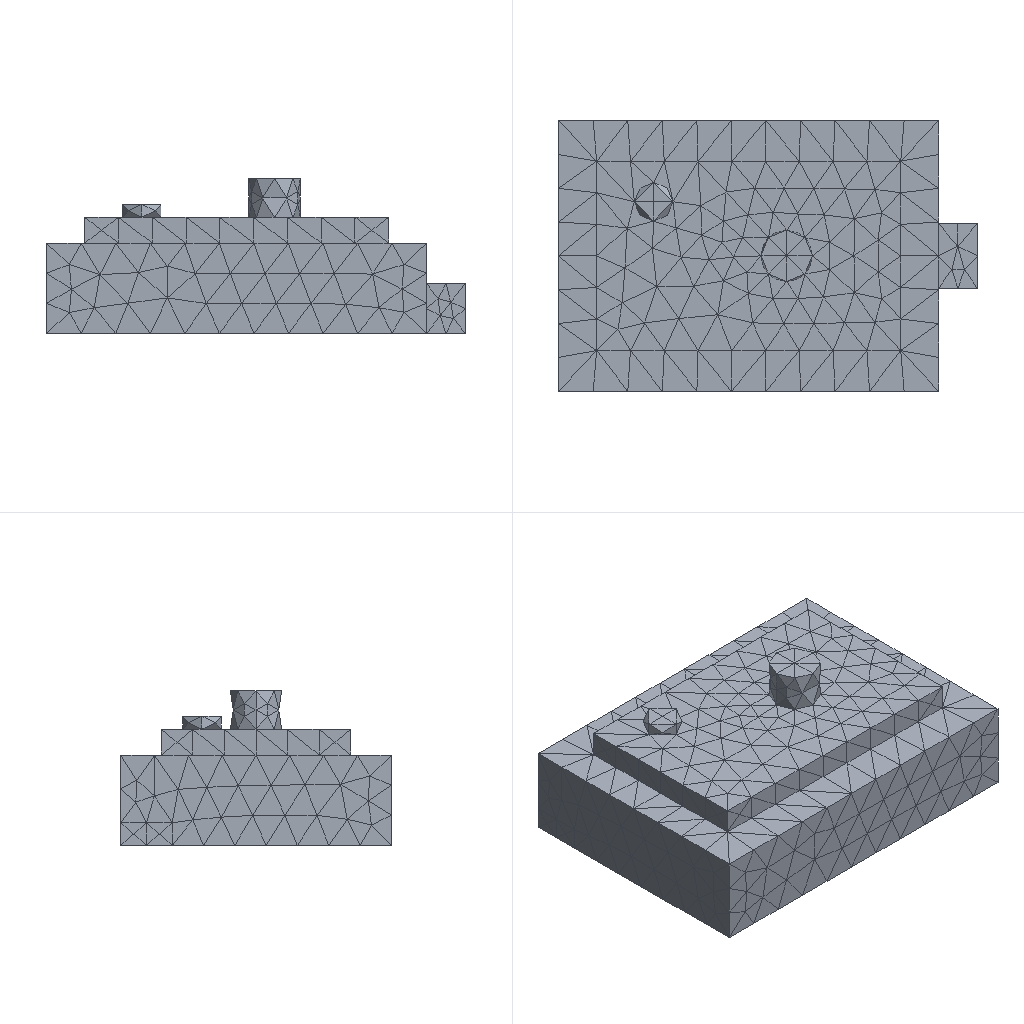Simulation study | ansys mapdl
Set-up summary:
category,name,step,type,value,unit,region
solver,ansys_mapdl
units,mm-N-s-tonne (MPa),,inferred,E=210000 density=
analysis,model,,static
mesh,nodes,,,5151
mesh,elements,,,3114
element_type,SOLID187,,,3114
material,mat 1,,E,210000
material,mat 1,,nu,0.3
load,,model,body load temp,,,all
load,,model,force,"1000 [dir=(0, 0, -1) n=162]",,node list
bc,,model,fixed,"[dofs=UX,UY,UZ n=5109]",,node list
Ansys APDL input file, long lists of numbers shortened:
/COM,ANSYS RELEASE 2026 R1           BUILD 26.1      UP20260202       09:08:46
/PREP7
/NOPR
/TITLE,2
ANTYPE, 0
*IF,_CDRDOFF,EQ,1,THEN     !if solid model was read in
_CDRDOFF=             !reset flag, numoffs already performed
*ELSE              !offset database for the following FE model
NUMOFF,NODE,     5151
NUMOFF,ELEM,     3114
NUMOFF,MAT ,        1
NUMOFF,TYPE,        1
*ENDIF
*SET,_RETURN ,  0.
*SET,_STATUS ,  0.
*SET,_UIQR   ,  162.
*SET,__FLOATPARAMETER__,  5151.
DOF,DELETE
ETBLOCK,        1,        1
(2i9,19a9)
        1      187        0        0        0        0        0        0        0        0        0        0        0        0        0        0        0        0        0        0        0
       -1
NBLOCK,6,SOLID,      5151,      5151
(3i9,6e21.13e3)
        1        0        0-4.3000000000000E+001 4.2000000000000E+001 7.0000000000000E+000
! (5150 more lines like these left out)
N,UNBL,LOC,       -1,
EBLOCK,19,SOLID,      3114,      3114
(19i10)
         1         1         1         1         0         0         0         0        10         0         1      1907      1650      1660      1649      2210      1327      2211      2212
! (6227 more lines like these left out)
        -1
MPTEMP,UNBL, 1, 1,  0.    ,
MPDATA,UNBL, 1,EX  ,       1, 1,  210000.000    ,
MPTEMP,UNBL, 1, 1,  0.    ,
MPDATA,UNBL, 1,NUXY,       1, 1, 0.3    ,
MPTEMP,UNBL, 1, 1,  0.    ,
MPDATA,UNBL, 1,PRXY,       1, 1, 0.3    ,
EXTOPT,ATTR,      0,      0,      0
EXTOPT,ESIZE,  0,  0.
EXTOPT,ACLEAR,      0
TREF,  0.
IRLF,  0
BFUNIF,TEMP,_TINY
ACEL,  0.    ,  0.    ,  0.
OMEGA,  0.    ,  0.    ,  0.
DOMEGA,  0.    ,  0.    ,  0.
CGLOC,  0.    ,  0.    ,  0.
CGOMEGA,  0.    ,  0.    ,  0.
DCGOMG,  0.    ,  0.    ,  0.
KUSE,     0
TIME,  0.
ALPHAD,  0.
BETAD,  0.
DMPRAT,  0.
DMPSTR,  0.
CRPLIM, 0.1    ,   0
CRPLIM,  0.    ,   1
NCNV,     0, 1.000000000E+12,     0,  0.    ,  0.
NEQIT,     0
ERESX,DEFA
DBLOCK,      5109
(i9,a6,2(pg16.9))
        1  UX    0.00000000      0.00000000
! (5108 more lines like these left out)
       -1
FBLOCK,       162
(i9,a6,2(pg16.9))
      910  FZ   -6.17283951      0.00000000
! (161 more lines like these left out)
       -1
/GO
FINISH
Results summary:
result,analysis_type_db,,,static,unstated
result,n_sets,,,1,unstated
result,load_steps[0].set,load_step=1,,1,unstated
result,load_steps[0].substep,load_step=1,,1,unstated
result,load_steps[0].time,load_step=1,,1,unstated
result,load_steps[0].freq,load_step=1,,1,unstated
result,load_steps[0].max_usum,load_step=1,,0.0004175,unstated
result,load_steps[0].max_seqv,load_step=1,,5.76,unstated
result,load_steps[0].reaction_sum.FX,load_step=1,,1.32627e-12,unstated
result,load_steps[0].reaction_sum.FY,load_step=1,,-2.52548e-13,unstated
result,load_steps[0].reaction_sum.FZ,load_step=1,,1000,unstated
result,load_steps[0].reaction_sum.MX,load_step=1,,0,unstated
result,load_steps[0].reaction_sum.MY,load_step=1,,0,unstated
result,load_steps[0].reaction_sum.MZ,load_step=1,,0,unstated
result,convergence,,,results present for all listed sets,unstated